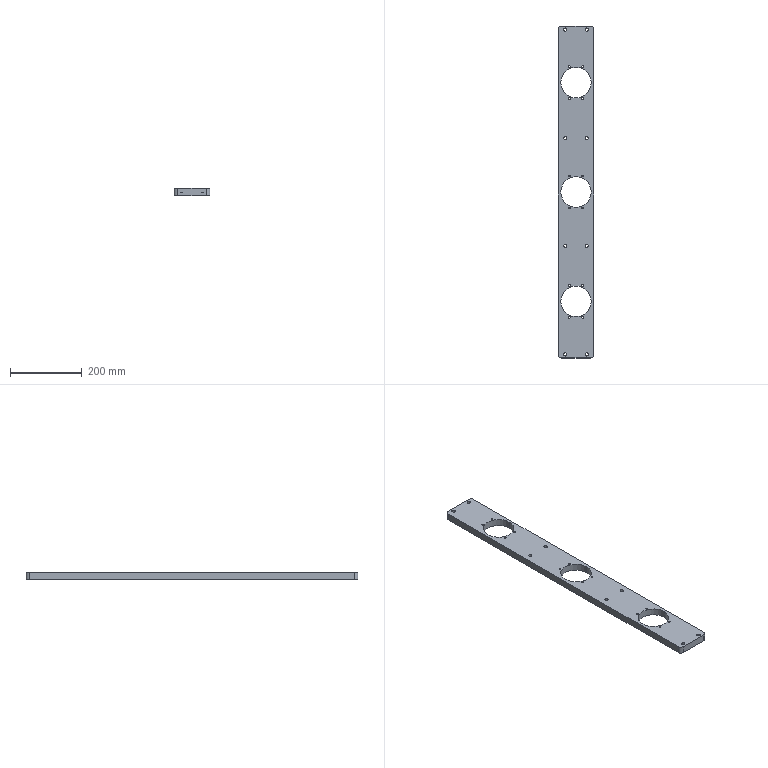Part | SolidWorks | features HoleWzd 3, ICE 2, Extrusion 1, Fillet 1, MirrorPattern 1 | 1 solid | 80 faces | box 100 x 925 x 20 mm | volume 1485141 mm3 | cylinder 66 | plane 14 | commonest cylinder face diameters 5 x24 9 x16 15 x16 85 x6 20 x4